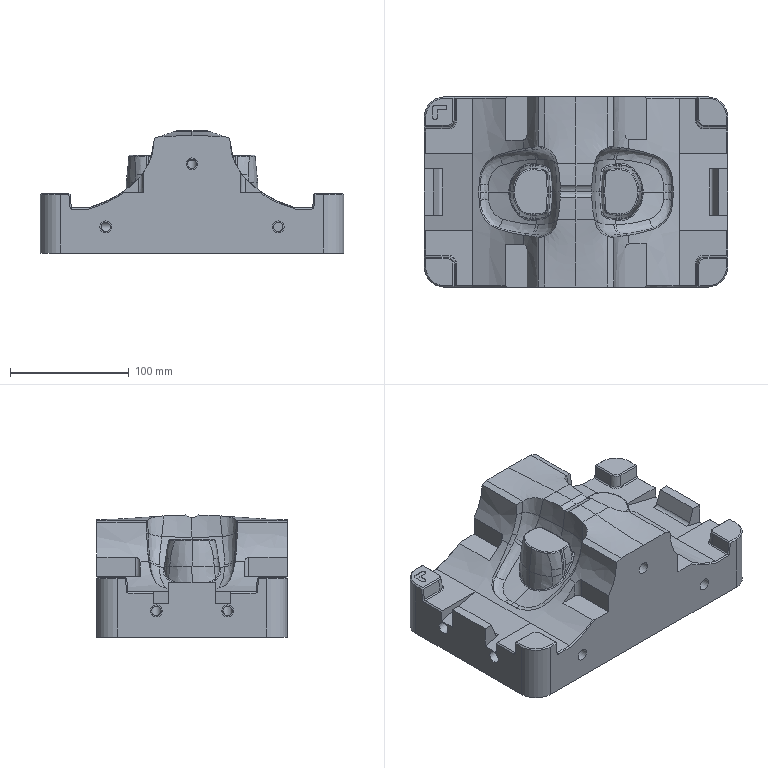CAM job | NX | 3-axis milling | part box 255 x 160 x 102.619 mm | stock box 255 x 160.003 x 102.62 mm
Tools:
number,name,description,diameter,corner_radius,flute_length,length,flutes
0,D30R5,Milling Tool-5 Parameters,30.0,5.0,50.0,75.0,2
0,D10,Milling Tool-5 Parameters,10.0,0.0,50.0,75.0,2
0,D8,Milling Tool-5 Parameters,8.0,0.0,50.0,75.0,2
0,BB6R3,Milling Tool-Ball Mill,6.0,3.0,50.0,75.0,2
Operations:
program,operation,operation_type,tool,method,geometry_group,spindle_rpm,surface_speed,feed_per_tooth,feed_cut,feed_plunge,cut_length_mm,path_length_mm,cut_time_min,machine_time_min
9-22_X_T01,CAVITY_MILL,CavityMilling,D30R5,METHOD,WORKPIECE,1500.0,141.0,0.6,1800.0,100.0,298335.66,301554.094,165.742,166.064
9-22_X_T01,ZLEVEL_PROFILE_COPY,ZLevelMilling,D30R5,METHOD,WORKPIECE,1500.0,37.0,0.6667,2000.0,100.0,30009.51,31232.59,15.005,15.127
9-22_X_T02,CAVITY_MILL_COPY,CavityMilling,D10,METHOD,WORKPIECE,1500.0,141.0,0.6,1800.0,100.0,33332.278,37138.238,18.518,18.898
9-22_X_T02,CAVITY_MILL_COPY_COPY,CavityMilling,D10,METHOD,WORKPIECE,1500.0,141.0,0.6,1800.0,100.0,33344.4,37163.326,18.525,18.907
9-22_X_T02,ZLEVEL_PROFILE_COPY_COPY,ZLevelMilling,D10,METHOD,WORKPIECE,1500.0,37.0,0.6667,2000.0,100.0,2830.514,4266.905,1.415,1.559
9-22_X_T02,ZLEVEL_PROFILE_COPY_COPY_COPY,ZLevelMilling,D10,METHOD,WORKPIECE,1500.0,37.0,0.6667,2000.0,100.0,22895.084,24140.453,11.447,11.572
9-22_X_T03,ZLEVEL_PROFILE,ZLevelMilling,D8,METHOD,WORKPIECE,3000.0,75.0,0.3,1800.0,100.0,54703.895,57609.373,30.391,30.682
9-22_X_T03,ZLEVEL_PROFILE_COPY_1,ZLevelMilling,D8,METHOD,WORKPIECE,3000.0,75.0,0.3,1800.0,100.0,54790.672,57500.978,30.439,30.71
9-22_X_T03,ZLEVEL_PROFILE_COPY_1_COPY,ZLevelMilling,D8,METHOD,WORKPIECE,3000.0,75.0,0.3,1800.0,100.0,2775.948,3277.266,1.542,1.592
9-22_X_T03,FACE_MILLING,FaceMilling,D8,METHOD,WORKPIECE,2000.0,50.0,0.2,800.0,100.0,3845.076,6355.491,4.806,5.057
9-22_X_T03,ZLEVEL_PROFILE_1,ZLevelMilling,D8,METHOD,WORKPIECE,3000.0,282.0,0.4167,2500.0,100.0,28498.887,30574.807,11.4,11.607
9-22_X_T04,ZLEVEL_PROFILE_2,ZLevelMilling,BB6R3,METHOD,WORKPIECE,3000.0,282.0,0.3,1800.0,100.0,11743.815,11899.083,6.524,6.54
9-22_X_T04,ZLEVEL_PROFILE_2_COPY,ZLevelMilling,BB6R3,METHOD,WORKPIECE,3000.0,282.0,0.3,1800.0,100.0,4854.463,5007.169,2.697,2.712
9-22_X_T04,ZLEVEL_PROFILE_2_COPY_COPY,ZLevelMilling,BB6R3,METHOD,WORKPIECE,3000.0,282.0,0.3,1800.0,100.0,4870.223,5021.705,2.706,2.721
9-22_X_T04,ZLEVEL_PROFILE_2_COPY_1,ZLevelMilling,BB6R3,METHOD,WORKPIECE,3000.0,282.0,0.3,1800.0,100.0,11729.034,11931.83,6.516,6.536
9-22_X_T04,FIXED_CONTOUR,SurfaceContour,BB6R3,METHOD,WORKPIECE,14961.0,282.0,0.0602,1800.0,100.0,17391.75,17713.526,9.662,9.694